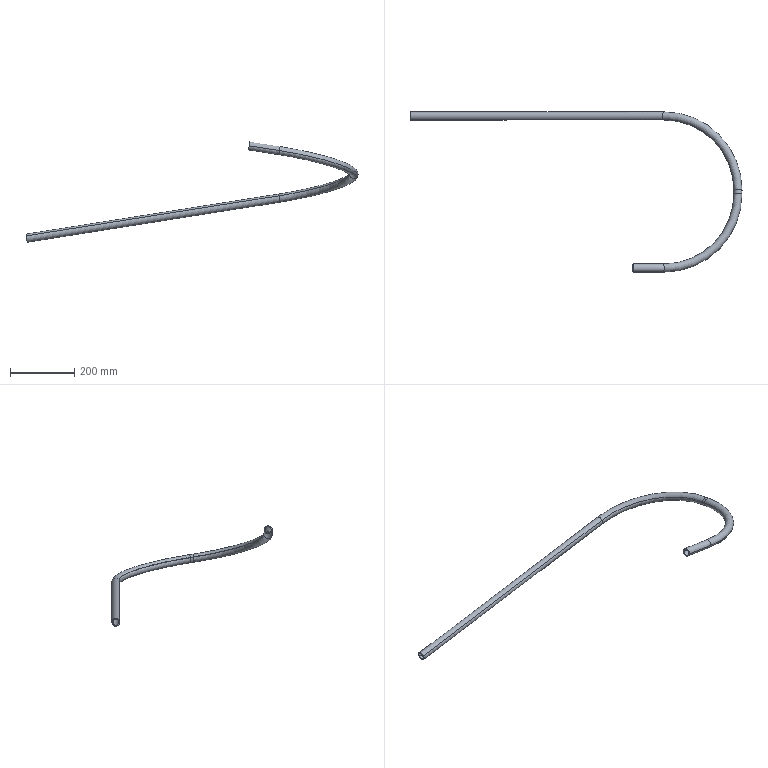Part | STEP file | 31E-01143WG10 | 1 solid | 22 faces | box 1031 x 498.4 x 311.784 mm | volume 326544 mm3 | cylinder 12 | torus 8 | plane 2 | commonest cylinder face diameters 19.8 x6 25.4 x6
STEP:
#1=CARTESIAN_POINT('',(-1196.479,198.036,1339.737));
#2=VERTEX_POINT('',#1);
#3=CARTESIAN_POINT('',(-411.266,198.036,1464.102));
#4=VERTEX_POINT('',#3);
#5=CARTESIAN_POINT('',(-427.761,198.036,1461.49));
#6=DIRECTION('',(0.9877,0.,0.1564));
#7=VECTOR('',#6,1.);
#8=LINE('',#5,#7);
#9=EDGE_CURVE('',#2,#4,#8,.T.);
#10=ORIENTED_EDGE('',*,*,#9,.F.);
#11=CARTESIAN_POINT('',(-1194.685,214.176,1328.409));
#12=VERTEX_POINT('',#11);
#13=CARTESIAN_POINT('',(-1195.582,206.106,1334.073));
#14=DIRECTION('',(0.9877,0.,0.1564));
#15=AXIS2_PLACEMENT_3D('',#13,#14,$);
#16=CIRCLE('',#15,9.9);
#17=EDGE_CURVE('',#2,#12,#16,.F.);
#18=ORIENTED_EDGE('',*,*,#17,.T.);
#19=CARTESIAN_POINT('',(-409.472,214.176,1452.774));
#20=VERTEX_POINT('',#19);
#21=CARTESIAN_POINT('',(-425.967,214.176,1450.162));
#22=DIRECTION('',(0.9877,0.,0.1564));
#23=VECTOR('',#22,1.);
#24=LINE('',#21,#23);
#25=EDGE_CURVE('',#12,#20,#24,.T.);
#26=ORIENTED_EDGE('',*,*,#25,.T.);
#27=CARTESIAN_POINT('',(-410.369,206.106,1458.438));
#28=DIRECTION('',(0.9877,0.,0.1564));
#29=AXIS2_PLACEMENT_3D('',#27,#28,$);
#30=CIRCLE('',#29,9.9);
#31=EDGE_CURVE('',#20,#4,#30,.T.);
#32=ORIENTED_EDGE('',*,*,#31,.T.);
#33=EDGE_LOOP('',(#10,#18,#26,#32));
#34=FACE_OUTER_BOUND('',#33,.T.);
#35=CARTESIAN_POINT('',(-426.864,206.106,1455.826));
#36=DIRECTION('',(0.9877,0.,0.1564));
#37=DIRECTION('',(0.09062,0.8151,-0.5721));
#38=AXIS2_PLACEMENT_3D('',#35,#36,#37);
#39=CYLINDRICAL_SURFACE('',#38,9.9);
#40=ADVANCED_FACE('',(#34),#39,.F.);
#41=CARTESIAN_POINT('',(-169.572,-25.868,1528.434));
#42=VERTEX_POINT('',#41);
#43=CARTESIAN_POINT('',(-415.434,-31.741,1490.415));
#44=DIRECTION('',(-0.1546,0.1531,0.976));
#45=AXIS2_PLACEMENT_3D('',#43,#44,$);
#46=CIRCLE('',#45,248.853);
#47=EDGE_CURVE('',#42,#20,#46,.T.);
#48=ORIENTED_EDGE('',*,*,#47,.F.);
#49=CARTESIAN_POINT('',(-188.435,-24.929,1534.379));
#50=VERTEX_POINT('',#49);
#51=CARTESIAN_POINT('',(-179.004,-25.399,1531.407));
#52=DIRECTION('',(-0.0003622,-0.9879,0.155));
#53=AXIS2_PLACEMENT_3D('',#51,#52,$);
#54=CIRCLE('',#53,9.9);
#55=EDGE_CURVE('',#42,#50,#54,.T.);
#56=ORIENTED_EDGE('',*,*,#55,.T.);
#57=CARTESIAN_POINT('',(-416.804,-30.384,1499.065));
#58=DIRECTION('',(-0.1546,0.1531,0.976));
#59=AXIS2_PLACEMENT_3D('',#57,#58,$);
#60=CIRCLE('',#59,231.147);
#61=EDGE_CURVE('',#50,#4,#60,.T.);
#62=ORIENTED_EDGE('',*,*,#61,.T.);
#63=ORIENTED_EDGE('',*,*,#31,.F.);
#64=EDGE_LOOP('',(#48,#56,#62,#63));
#65=FACE_OUTER_BOUND('',#64,.T.);
#66=CARTESIAN_POINT('',(-416.119,-31.063,1494.74));
#67=DIRECTION('',(-0.1546,0.1531,0.976));
#68=DIRECTION('',(0.988,0.0236,0.1528));
#69=AXIS2_PLACEMENT_3D('',#66,#67,#68);
#70=TOROIDAL_SURFACE('',#69,240.,9.9);
#71=ADVANCED_FACE('',(#65),#70,.F.);
#72=CARTESIAN_POINT('',(-169.576,-36.024,1530.027));
#73=VERTEX_POINT('',#72);
#74=CARTESIAN_POINT('',(-169.574,-30.946,1529.231));
#75=DIRECTION('',(-0.0003622,-0.9879,0.155));
#76=VECTOR('',#75,1.);
#77=LINE('',#74,#76);
#78=EDGE_CURVE('',#73,#42,#77,.F.);
#79=ORIENTED_EDGE('',*,*,#78,.F.);
#80=CARTESIAN_POINT('',(-188.439,-35.085,1535.972));
#81=VERTEX_POINT('',#80);
#82=CARTESIAN_POINT('',(-179.007,-35.555,1533.));
#83=DIRECTION('',(-0.0003622,-0.9879,0.155));
#84=AXIS2_PLACEMENT_3D('',#82,#83,$);
#85=CIRCLE('',#84,9.9);
#86=EDGE_CURVE('',#73,#81,#85,.T.);
#87=ORIENTED_EDGE('',*,*,#86,.T.);
#88=CARTESIAN_POINT('',(-188.437,-30.007,1535.176));
#89=DIRECTION('',(-0.0003622,-0.9879,0.155));
#90=VECTOR('',#89,1.);
#91=LINE('',#88,#90);
#92=EDGE_CURVE('',#81,#50,#91,.F.);
#93=ORIENTED_EDGE('',*,*,#92,.T.);
#94=ORIENTED_EDGE('',*,*,#55,.F.);
#95=EDGE_LOOP('',(#79,#87,#93,#94));
#96=FACE_OUTER_BOUND('',#95,.T.);
#97=CARTESIAN_POINT('',(-179.006,-30.477,1532.203));
#98=DIRECTION('',(-0.0003622,-0.9879,0.155));
#99=DIRECTION('',(0.9527,-0.04744,-0.3002));
#100=AXIS2_PLACEMENT_3D('',#97,#98,#99);
#101=CYLINDRICAL_SURFACE('',#100,9.9);
#102=ADVANCED_FACE('',(#96),#101,.F.);
#103=ORIENTED_EDGE('',*,*,#92,.F.);
#104=CARTESIAN_POINT('',(-179.007,-35.555,1533.));
#105=DIRECTION('',(-0.0003622,-0.9879,0.155));
#106=AXIS2_PLACEMENT_3D('',#104,#105,$);
#107=CIRCLE('',#106,9.9);
#108=EDGE_CURVE('',#81,#73,#107,.T.);
#109=ORIENTED_EDGE('',*,*,#108,.T.);
#110=ORIENTED_EDGE('',*,*,#78,.T.);
#111=CARTESIAN_POINT('',(-179.004,-25.399,1531.407));
#112=DIRECTION('',(-0.0003622,-0.9879,0.155));
#113=AXIS2_PLACEMENT_3D('',#111,#112,$);
#114=CIRCLE('',#113,9.9);
#115=EDGE_CURVE('',#50,#42,#114,.T.);
#116=ORIENTED_EDGE('',*,*,#115,.F.);
#117=EDGE_LOOP('',(#103,#109,#110,#116));
#118=FACE_OUTER_BOUND('',#117,.T.);
#119=CARTESIAN_POINT('',(-179.006,-30.477,1532.203));
#120=DIRECTION('',(-0.0003622,-0.9879,0.155));
#121=DIRECTION('',(-0.9527,0.04744,0.3002));
#122=AXIS2_PLACEMENT_3D('',#119,#120,#121);
#123=CYLINDRICAL_SURFACE('',#122,9.9);
#124=ADVANCED_FACE('',(#118),#123,.F.);
#125=CARTESIAN_POINT('',(-410.377,-256.994,1605.916));
#126=VERTEX_POINT('',#125);
#127=CARTESIAN_POINT('',(-410.377,-276.794,1605.916));
#128=VERTEX_POINT('',#127);
#129=CARTESIAN_POINT('',(-410.377,-266.894,1605.916));
#130=DIRECTION('',(0.9877,0.,-0.1564));
#131=AXIS2_PLACEMENT_3D('',#129,#130,$);
#132=CIRCLE('',#131,9.9);
#133=EDGE_CURVE('',#126,#128,#132,.F.);
#134=ORIENTED_EDGE('',*,*,#133,.T.);
#135=CARTESIAN_POINT('',(-416.356,-29.953,1568.162));
#136=DIRECTION('',(-0.1546,-0.153,-0.9761));
#137=AXIS2_PLACEMENT_3D('',#135,#136,$);
#138=CIRCLE('',#137,249.783);
#139=EDGE_CURVE('',#73,#128,#138,.T.);
#140=ORIENTED_EDGE('',*,*,#139,.F.);
#141=ORIENTED_EDGE('',*,*,#108,.F.);
#142=CARTESIAN_POINT('',(-415.888,-29.489,1571.119));
#143=DIRECTION('',(-0.1546,-0.153,-0.9761));
#144=AXIS2_PLACEMENT_3D('',#142,#143,$);
#145=CIRCLE('',#144,230.217);
#146=EDGE_CURVE('',#81,#126,#145,.T.);
#147=ORIENTED_EDGE('',*,*,#146,.T.);
#148=EDGE_LOOP('',(#134,#140,#141,#147));
#149=FACE_OUTER_BOUND('',#148,.T.);
#150=CARTESIAN_POINT('',(-416.122,-29.721,1569.64));
#151=DIRECTION('',(-0.1546,-0.153,-0.9761));
#152=DIRECTION('',(0.988,-0.02431,-0.1527));
#153=AXIS2_PLACEMENT_3D('',#150,#151,#152);
#154=TOROIDAL_SURFACE('',#153,240.,9.9);
#155=ADVANCED_FACE('',(#149),#154,.F.);
#156=CARTESIAN_POINT('',(-410.377,-266.894,1605.916));
#157=DIRECTION('',(0.9877,0.,-0.1564));
#158=AXIS2_PLACEMENT_3D('',#156,#157,$);
#159=CIRCLE('',#158,9.9);
#160=EDGE_CURVE('',#128,#126,#159,.F.);
#161=ORIENTED_EDGE('',*,*,#160,.T.);
#162=ORIENTED_EDGE('',*,*,#146,.F.);
#163=ORIENTED_EDGE('',*,*,#86,.F.);
#164=ORIENTED_EDGE('',*,*,#139,.T.);
#165=EDGE_LOOP('',(#161,#162,#163,#164));
#166=FACE_OUTER_BOUND('',#165,.T.);
#167=CARTESIAN_POINT('',(-416.122,-29.721,1569.64));
#168=DIRECTION('',(-0.1546,-0.153,-0.9761));
#169=DIRECTION('',(0.988,-0.02431,-0.1527));
#170=AXIS2_PLACEMENT_3D('',#167,#168,#169);
#171=TOROIDAL_SURFACE('',#170,240.,9.9);
#172=ADVANCED_FACE('',(#166),#171,.F.);
#173=CARTESIAN_POINT('',(-504.155,-276.794,1620.769));
#174=VERTEX_POINT('',#173);
#175=CARTESIAN_POINT('',(-433.907,-276.794,1609.643));
#176=DIRECTION('',(-0.9877,0.,0.1564));
#177=VECTOR('',#176,1.);
#178=LINE('',#175,#177);
#179=EDGE_CURVE('',#128,#174,#178,.T.);
#180=ORIENTED_EDGE('',*,*,#179,.T.);
#181=CARTESIAN_POINT('',(-504.155,-256.994,1620.769));
#182=VERTEX_POINT('',#181);
#183=CARTESIAN_POINT('',(-504.155,-266.894,1620.769));
#184=DIRECTION('',(-0.9877,0.,0.1564));
#185=AXIS2_PLACEMENT_3D('',#183,#184,$);
#186=CIRCLE('',#185,9.9);
#187=EDGE_CURVE('',#174,#182,#186,.T.);
#188=ORIENTED_EDGE('',*,*,#187,.T.);
#189=CARTESIAN_POINT('',(-433.907,-256.994,1609.643));
#190=DIRECTION('',(-0.9877,0.,0.1564));
#191=VECTOR('',#190,1.);
#192=LINE('',#189,#191);
#193=EDGE_CURVE('',#126,#182,#192,.T.);
#194=ORIENTED_EDGE('',*,*,#193,.F.);
#195=ORIENTED_EDGE('',*,*,#160,.F.);
#196=EDGE_LOOP('',(#180,#188,#194,#195));
#197=FACE_OUTER_BOUND('',#196,.T.);
#198=CARTESIAN_POINT('',(-433.907,-266.894,1609.643));
#199=DIRECTION('',(-0.9877,0.,0.1564));
#200=DIRECTION('',(0.,-1.,0.));
#201=AXIS2_PLACEMENT_3D('',#198,#199,#200);
#202=CYLINDRICAL_SURFACE('',#201,9.9);
#203=ADVANCED_FACE('',(#197),#202,.F.);
#204=CARTESIAN_POINT('',(-504.155,-266.894,1620.769));
#205=DIRECTION('',(-0.9877,0.,0.1564));
#206=AXIS2_PLACEMENT_3D('',#204,#205,$);
#207=CIRCLE('',#206,9.9);
#208=EDGE_CURVE('',#182,#174,#207,.T.);
#209=ORIENTED_EDGE('',*,*,#208,.T.);
#210=ORIENTED_EDGE('',*,*,#179,.F.);
#211=ORIENTED_EDGE('',*,*,#133,.F.);
#212=ORIENTED_EDGE('',*,*,#193,.T.);
#213=EDGE_LOOP('',(#209,#210,#211,#212));
#214=FACE_OUTER_BOUND('',#213,.T.);
#215=CARTESIAN_POINT('',(-433.907,-266.894,1609.643));
#216=DIRECTION('',(-0.9877,0.,0.1564));
#217=DIRECTION('',(0.,1.,0.));
#218=AXIS2_PLACEMENT_3D('',#215,#216,#217);
#219=CYLINDRICAL_SURFACE('',#218,9.9);
#220=ADVANCED_FACE('',(#214),#219,.F.);
#221=CARTESIAN_POINT('',(-504.155,-254.194,1620.769));
#222=VERTEX_POINT('',#221);
#223=CARTESIAN_POINT('',(-504.155,-279.594,1620.769));
#224=VERTEX_POINT('',#223);
#225=CARTESIAN_POINT('',(-504.155,-279.594,1620.769));
#226=CARTESIAN_POINT('',(-504.467,-279.594,1618.799));
#227=CARTESIAN_POINT('',(-504.779,-279.202,1616.828));
#228=CARTESIAN_POINT('',(-505.075,-278.418,1614.959));
#229=CARTESIAN_POINT('',(-505.603,-276.151,1611.626));
#230=CARTESIAN_POINT('',(-505.958,-272.776,1609.386));
#231=CARTESIAN_POINT('',(-506.081,-270.884,1608.612));
#232=CARTESIAN_POINT('',(-506.203,-266.894,1607.839));
#233=CARTESIAN_POINT('',(-506.081,-262.904,1608.612));
#234=CARTESIAN_POINT('',(-505.958,-261.012,1609.386));
#235=CARTESIAN_POINT('',(-505.603,-257.637,1611.626));
#236=CARTESIAN_POINT('',(-505.075,-255.369,1614.959));
#237=CARTESIAN_POINT('',(-504.779,-254.586,1616.828));
#238=CARTESIAN_POINT('',(-504.467,-254.194,1618.799));
#239=CARTESIAN_POINT('',(-504.155,-254.194,1620.769));
#240=B_SPLINE_CURVE_WITH_KNOTS('',5,(#225,#226,#227,#228,#229,#230,#231,#232,#233,#234,#235,#236,#237,#238,#239),.UNSPECIFIED.,.F.,.U.,(6,3,3,3,6),(39.898,49.873,59.847,69.822,79.796),.UNSPECIFIED.);
#241=EDGE_CURVE('',#222,#224,#240,.F.);
#242=ORIENTED_EDGE('',*,*,#241,.T.);
#243=CARTESIAN_POINT('',(-504.155,-254.194,1620.769));
#244=CARTESIAN_POINT('',(-503.843,-254.194,1622.739));
#245=CARTESIAN_POINT('',(-503.531,-254.586,1624.71));
#246=CARTESIAN_POINT('',(-503.235,-255.369,1626.579));
#247=CARTESIAN_POINT('',(-502.707,-257.637,1629.912));
#248=CARTESIAN_POINT('',(-502.352,-261.012,1632.152));
#249=CARTESIAN_POINT('',(-502.23,-262.904,1632.926));
#250=CARTESIAN_POINT('',(-502.107,-266.894,1633.7));
#251=CARTESIAN_POINT('',(-502.23,-270.884,1632.926));
#252=CARTESIAN_POINT('',(-502.352,-272.776,1632.152));
#253=CARTESIAN_POINT('',(-502.707,-276.151,1629.912));
#254=CARTESIAN_POINT('',(-503.235,-278.418,1626.579));
#255=CARTESIAN_POINT('',(-503.531,-279.202,1624.71));
#256=CARTESIAN_POINT('',(-503.843,-279.594,1622.739));
#257=CARTESIAN_POINT('',(-504.155,-279.594,1620.769));
#258=B_SPLINE_CURVE_WITH_KNOTS('',5,(#243,#244,#245,#246,#247,#248,#249,#250,#251,#252,#253,#254,#255,#256,#257),.UNSPECIFIED.,.F.,.U.,(6,3,3,3,6),(0.,9.975,19.949,29.924,39.898),.UNSPECIFIED.);
#259=EDGE_CURVE('',#224,#222,#258,.F.);
#260=ORIENTED_EDGE('',*,*,#259,.T.);
#261=EDGE_LOOP('',(#242,#260));
#262=FACE_OUTER_BOUND('',#261,.T.);
#263=ORIENTED_EDGE('',*,*,#208,.F.);
#264=ORIENTED_EDGE('',*,*,#187,.F.);
#265=EDGE_LOOP('',(#263,#264));
#266=FACE_BOUND('',#265,.T.);
#267=CARTESIAN_POINT('',(-504.155,-266.894,1620.769));
#268=DIRECTION('',(0.9877,0.,-0.1564));
#269=DIRECTION('',(0.,1.,0.));
#270=AXIS2_PLACEMENT_3D('',#267,#268,#269);
#271=PLANE('',#270);
#272=ADVANCED_FACE('',(#262,#266),#271,.F.);
#273=CARTESIAN_POINT('',(-410.377,-279.594,1605.916));
#274=VERTEX_POINT('',#273);
#275=CARTESIAN_POINT('',(-433.907,-279.594,1609.643));
#276=DIRECTION('',(-0.9877,0.,0.1564));
#277=VECTOR('',#276,1.);
#278=LINE('',#275,#277);
#279=EDGE_CURVE('',#274,#224,#278,.T.);
#280=ORIENTED_EDGE('',*,*,#279,.F.);
#281=CARTESIAN_POINT('',(-410.377,-254.194,1605.916));
#282=VERTEX_POINT('',#281);
#283=CARTESIAN_POINT('',(-410.377,-266.894,1605.916));
#284=DIRECTION('',(-0.9877,0.,0.1564));
#285=AXIS2_PLACEMENT_3D('',#283,#284,$);
#286=CIRCLE('',#285,12.7);
#287=EDGE_CURVE('',#274,#282,#286,.T.);
#288=ORIENTED_EDGE('',*,*,#287,.T.);
#289=CARTESIAN_POINT('',(-433.907,-254.194,1609.643));
#290=DIRECTION('',(-0.9877,0.,0.1564));
#291=VECTOR('',#290,1.);
#292=LINE('',#289,#291);
#293=EDGE_CURVE('',#282,#222,#292,.T.);
#294=ORIENTED_EDGE('',*,*,#293,.T.);
#295=ORIENTED_EDGE('',*,*,#259,.F.);
#296=EDGE_LOOP('',(#280,#288,#294,#295));
#297=FACE_OUTER_BOUND('',#296,.T.);
#298=CARTESIAN_POINT('',(-433.907,-266.894,1609.643));
#299=DIRECTION('',(-0.9877,0.,0.1564));
#300=DIRECTION('',(0.,-1.,0.));
#301=AXIS2_PLACEMENT_3D('',#298,#299,#300);
#302=CYLINDRICAL_SURFACE('',#301,12.7);
#303=ADVANCED_FACE('',(#297),#302,.T.);
#304=CARTESIAN_POINT('',(-166.908,-36.157,1529.187));
#305=VERTEX_POINT('',#304);
#306=CARTESIAN_POINT('',(-416.423,-30.018,1567.743));
#307=DIRECTION('',(-0.1546,-0.153,-0.9761));
#308=AXIS2_PLACEMENT_3D('',#306,#307,$);
#309=CIRCLE('',#308,252.55);
#310=EDGE_CURVE('',#305,#274,#309,.T.);
#311=ORIENTED_EDGE('',*,*,#310,.F.);
#312=CARTESIAN_POINT('',(-191.107,-34.952,1536.813));
#313=VERTEX_POINT('',#312);
#314=CARTESIAN_POINT('',(-179.007,-35.555,1533.));
#315=DIRECTION('',(0.0003622,0.9879,-0.155));
#316=AXIS2_PLACEMENT_3D('',#314,#315,$);
#317=CIRCLE('',#316,12.7);
#318=EDGE_CURVE('',#305,#313,#317,.F.);
#319=ORIENTED_EDGE('',*,*,#318,.T.);
#320=CARTESIAN_POINT('',(-415.822,-29.423,1571.537));
#321=DIRECTION('',(-0.1546,-0.153,-0.9761));
#322=AXIS2_PLACEMENT_3D('',#320,#321,$);
#323=CIRCLE('',#322,227.45);
#324=EDGE_CURVE('',#313,#282,#323,.T.);
#325=ORIENTED_EDGE('',*,*,#324,.T.);
#326=ORIENTED_EDGE('',*,*,#287,.F.);
#327=EDGE_LOOP('',(#311,#319,#325,#326));
#328=FACE_OUTER_BOUND('',#327,.T.);
#329=CARTESIAN_POINT('',(-416.122,-29.721,1569.64));
#330=DIRECTION('',(-0.1546,-0.153,-0.9761));
#331=DIRECTION('',(0.988,-0.02431,-0.1527));
#332=AXIS2_PLACEMENT_3D('',#329,#330,#331);
#333=TOROIDAL_SURFACE('',#332,240.,12.7);
#334=ADVANCED_FACE('',(#328),#333,.T.);
#335=CARTESIAN_POINT('',(-166.905,-26.001,1527.594));
#336=VERTEX_POINT('',#335);
#337=CARTESIAN_POINT('',(-191.103,-24.796,1535.22));
#338=VERTEX_POINT('',#337);
#339=CARTESIAN_POINT('',(-179.004,-25.399,1531.407));
#340=DIRECTION('',(-0.0003622,-0.9879,0.155));
#341=AXIS2_PLACEMENT_3D('',#339,#340,$);
#342=CIRCLE('',#341,12.7);
#343=EDGE_CURVE('',#336,#338,#342,.T.);
#344=ORIENTED_EDGE('',*,*,#343,.T.);
#345=CARTESIAN_POINT('',(-191.105,-29.874,1536.016));
#346=DIRECTION('',(-0.0003622,-0.9879,0.155));
#347=VECTOR('',#346,1.);
#348=LINE('',#345,#347);
#349=EDGE_CURVE('',#313,#338,#348,.F.);
#350=ORIENTED_EDGE('',*,*,#349,.F.);
#351=ORIENTED_EDGE('',*,*,#318,.F.);
#352=CARTESIAN_POINT('',(-166.906,-31.079,1528.39));
#353=DIRECTION('',(-0.0003622,-0.9879,0.155));
#354=VECTOR('',#353,1.);
#355=LINE('',#352,#354);
#356=EDGE_CURVE('',#305,#336,#355,.F.);
#357=ORIENTED_EDGE('',*,*,#356,.T.);
#358=EDGE_LOOP('',(#344,#350,#351,#357));
#359=FACE_OUTER_BOUND('',#358,.T.);
#360=CARTESIAN_POINT('',(-179.006,-30.477,1532.203));
#361=DIRECTION('',(-0.0003622,-0.9879,0.155));
#362=DIRECTION('',(0.9527,-0.04744,-0.3002));
#363=AXIS2_PLACEMENT_3D('',#360,#361,#362);
#364=CYLINDRICAL_SURFACE('',#363,12.7);
#365=ADVANCED_FACE('',(#359),#364,.T.);
#366=CARTESIAN_POINT('',(-179.004,-25.399,1531.407));
#367=DIRECTION('',(-0.0003622,-0.9879,0.155));
#368=AXIS2_PLACEMENT_3D('',#366,#367,$);
#369=CIRCLE('',#368,12.7);
#370=EDGE_CURVE('',#338,#336,#369,.T.);
#371=ORIENTED_EDGE('',*,*,#370,.T.);
#372=ORIENTED_EDGE('',*,*,#356,.F.);
#373=CARTESIAN_POINT('',(-179.007,-35.555,1533.));
#374=DIRECTION('',(-0.0003622,-0.9879,0.155));
#375=AXIS2_PLACEMENT_3D('',#373,#374,$);
#376=CIRCLE('',#375,12.7);
#377=EDGE_CURVE('',#313,#305,#376,.T.);
#378=ORIENTED_EDGE('',*,*,#377,.F.);
#379=ORIENTED_EDGE('',*,*,#349,.T.);
#380=EDGE_LOOP('',(#371,#372,#378,#379));
#381=FACE_OUTER_BOUND('',#380,.T.);
#382=CARTESIAN_POINT('',(-179.006,-30.477,1532.203));
#383=DIRECTION('',(-0.0003622,-0.9879,0.155));
#384=DIRECTION('',(-0.9527,0.04744,0.3002));
#385=AXIS2_PLACEMENT_3D('',#382,#383,#384);
#386=CYLINDRICAL_SURFACE('',#385,12.7);
#387=ADVANCED_FACE('',(#381),#386,.T.);
#388=ORIENTED_EDGE('',*,*,#324,.F.);
#389=ORIENTED_EDGE('',*,*,#377,.T.);
#390=ORIENTED_EDGE('',*,*,#310,.T.);
#391=CARTESIAN_POINT('',(-410.377,-266.894,1605.916));
#392=DIRECTION('',(0.9877,0.,-0.1564));
#393=AXIS2_PLACEMENT_3D('',#391,#392,$);
#394=CIRCLE('',#393,12.7);
#395=EDGE_CURVE('',#282,#274,#394,.F.);
#396=ORIENTED_EDGE('',*,*,#395,.F.);
#397=EDGE_LOOP('',(#388,#389,#390,#396));
#398=FACE_OUTER_BOUND('',#397,.T.);
#399=CARTESIAN_POINT('',(-416.122,-29.721,1569.64));
#400=DIRECTION('',(-0.1546,-0.153,-0.9761));
#401=DIRECTION('',(0.988,-0.02431,-0.1527));
#402=AXIS2_PLACEMENT_3D('',#399,#400,#401);
#403=TOROIDAL_SURFACE('',#402,240.,12.7);
#404=ADVANCED_FACE('',(#398),#403,.T.);
#405=ORIENTED_EDGE('',*,*,#279,.T.);
#406=ORIENTED_EDGE('',*,*,#241,.F.);
#407=ORIENTED_EDGE('',*,*,#293,.F.);
#408=ORIENTED_EDGE('',*,*,#395,.T.);
#409=EDGE_LOOP('',(#405,#406,#407,#408));
#410=FACE_OUTER_BOUND('',#409,.T.);
#411=CARTESIAN_POINT('',(-433.907,-266.894,1609.643));
#412=DIRECTION('',(-0.9877,0.,0.1564));
#413=DIRECTION('',(0.,1.,0.));
#414=AXIS2_PLACEMENT_3D('',#411,#412,#413);
#415=CYLINDRICAL_SURFACE('',#414,12.7);
#416=ADVANCED_FACE('',(#410),#415,.T.);
#417=CARTESIAN_POINT('',(-411.52,195.754,1465.704));
#418=VERTEX_POINT('',#417);
#419=CARTESIAN_POINT('',(-409.218,216.458,1451.172));
#420=VERTEX_POINT('',#419);
#421=CARTESIAN_POINT('',(-410.369,206.106,1458.438));
#422=DIRECTION('',(0.9877,0.,0.1564));
#423=AXIS2_PLACEMENT_3D('',#421,#422,$);
#424=CIRCLE('',#423,12.7);
#425=EDGE_CURVE('',#418,#420,#424,.T.);
#426=ORIENTED_EDGE('',*,*,#425,.T.);
#427=CARTESIAN_POINT('',(-415.24,-31.933,1489.192));
#428=DIRECTION('',(-0.1546,0.1531,0.976));
#429=AXIS2_PLACEMENT_3D('',#427,#428,$);
#430=CIRCLE('',#429,251.357);
#431=EDGE_CURVE('',#336,#420,#430,.T.);
#432=ORIENTED_EDGE('',*,*,#431,.F.);
#433=ORIENTED_EDGE('',*,*,#370,.F.);
#434=CARTESIAN_POINT('',(-416.997,-30.192,1500.288));
#435=DIRECTION('',(-0.1546,0.1531,0.976));
#436=AXIS2_PLACEMENT_3D('',#434,#435,$);
#437=CIRCLE('',#436,228.643);
#438=EDGE_CURVE('',#338,#418,#437,.T.);
#439=ORIENTED_EDGE('',*,*,#438,.T.);
#440=EDGE_LOOP('',(#426,#432,#433,#439));
#441=FACE_OUTER_BOUND('',#440,.T.);
#442=CARTESIAN_POINT('',(-416.119,-31.063,1494.74));
#443=DIRECTION('',(-0.1546,0.1531,0.976));
#444=DIRECTION('',(0.988,0.0236,0.1528));
#445=AXIS2_PLACEMENT_3D('',#442,#443,#444);
#446=TOROIDAL_SURFACE('',#445,240.,12.7);
#447=ADVANCED_FACE('',(#441),#446,.T.);
#448=CARTESIAN_POINT('',(-410.369,206.106,1458.438));
#449=DIRECTION('',(0.9877,0.,0.1564));
#450=AXIS2_PLACEMENT_3D('',#448,#449,$);
#451=CIRCLE('',#450,12.7);
#452=EDGE_CURVE('',#420,#418,#451,.T.);
#453=ORIENTED_EDGE('',*,*,#452,.T.);
#454=ORIENTED_EDGE('',*,*,#438,.F.);
#455=ORIENTED_EDGE('',*,*,#343,.F.);
#456=ORIENTED_EDGE('',*,*,#431,.T.);
#457=EDGE_LOOP('',(#453,#454,#455,#456));
#458=FACE_OUTER_BOUND('',#457,.T.);
#459=CARTESIAN_POINT('',(-416.119,-31.063,1494.74));
#460=DIRECTION('',(-0.1546,0.1531,0.976));
#461=DIRECTION('',(0.988,0.0236,0.1528));
#462=AXIS2_PLACEMENT_3D('',#459,#460,#461);
#463=TOROIDAL_SURFACE('',#462,240.,12.7);
#464=ADVANCED_FACE('',(#458),#463,.T.);
#465=ORIENTED_EDGE('',*,*,#452,.F.);
#466=CARTESIAN_POINT('',(-1194.431,216.458,1326.807));
#467=VERTEX_POINT('',#466);
#468=CARTESIAN_POINT('',(-425.713,216.458,1448.56));
#469=DIRECTION('',(0.9877,0.,0.1564));
#470=VECTOR('',#469,1.);
#471=LINE('',#468,#470);
#472=EDGE_CURVE('',#467,#420,#471,.T.);
#473=ORIENTED_EDGE('',*,*,#472,.F.);
#474=CARTESIAN_POINT('',(-1196.733,195.754,1341.339));
#475=VERTEX_POINT('',#474);
#476=CARTESIAN_POINT('',(-1195.582,206.106,1334.073));
#477=DIRECTION('',(0.9877,0.,0.1564));
#478=AXIS2_PLACEMENT_3D('',#476,#477,$);
#479=CIRCLE('',#478,12.7);
#480=EDGE_CURVE('',#475,#467,#479,.F.);
#481=ORIENTED_EDGE('',*,*,#480,.F.);
#482=CARTESIAN_POINT('',(-428.015,195.754,1463.092));
#483=DIRECTION('',(0.9877,0.,0.1564));
#484=VECTOR('',#483,1.);
#485=LINE('',#482,#484);
#486=EDGE_CURVE('',#475,#418,#485,.T.);
#487=ORIENTED_EDGE('',*,*,#486,.T.);
#488=EDGE_LOOP('',(#465,#473,#481,#487));
#489=FACE_OUTER_BOUND('',#488,.T.);
#490=CARTESIAN_POINT('',(-426.864,206.106,1455.826));
#491=DIRECTION('',(0.9877,0.,0.1564));
#492=DIRECTION('',(0.09062,0.8151,-0.5721));
#493=AXIS2_PLACEMENT_3D('',#490,#491,#492);
#494=CYLINDRICAL_SURFACE('',#493,12.7);
#495=ADVANCED_FACE('',(#489),#494,.T.);
#496=ORIENTED_EDGE('',*,*,#486,.F.);
#497=CARTESIAN_POINT('',(-1195.582,206.106,1334.073));
#498=DIRECTION('',(0.9877,0.,0.1564));
#499=AXIS2_PLACEMENT_3D('',#497,#498,$);
#500=CIRCLE('',#499,12.7);
#501=EDGE_CURVE('',#467,#475,#500,.F.);
#502=ORIENTED_EDGE('',*,*,#501,.F.);
#503=ORIENTED_EDGE('',*,*,#472,.T.);
#504=ORIENTED_EDGE('',*,*,#425,.F.);
#505=EDGE_LOOP('',(#496,#502,#503,#504));
#506=FACE_OUTER_BOUND('',#505,.T.);
#507=CARTESIAN_POINT('',(-426.864,206.106,1455.826));
#508=DIRECTION('',(0.9877,0.,0.1564));
#509=DIRECTION('',(-0.09062,-0.8151,0.5721));
#510=AXIS2_PLACEMENT_3D('',#507,#508,#509);
#511=CYLINDRICAL_SURFACE('',#510,12.7);
#512=ADVANCED_FACE('',(#506),#511,.T.);
#513=ORIENTED_EDGE('',*,*,#501,.T.);
#514=ORIENTED_EDGE('',*,*,#480,.T.);
#515=EDGE_LOOP('',(#513,#514));
#516=FACE_OUTER_BOUND('',#515,.T.);
#517=ORIENTED_EDGE('',*,*,#17,.F.);
#518=CARTESIAN_POINT('',(-1196.479,198.036,1339.737));
#519=CARTESIAN_POINT('',(-1196.281,197.135,1338.485));
#520=CARTESIAN_POINT('',(-1196.055,196.483,1337.058));
#521=CARTESIAN_POINT('',(-1195.811,196.127,1335.521));
#522=CARTESIAN_POINT('',(-1195.316,196.044,1332.391));
#523=CARTESIAN_POINT('',(-1194.852,197.165,1329.463));
#524=CARTESIAN_POINT('',(-1194.64,198.013,1328.127));
#525=CARTESIAN_POINT('',(-1194.281,200.195,1325.856));
#526=CARTESIAN_POINT('',(-1194.077,203.084,1324.569));
#527=CARTESIAN_POINT('',(-1194.021,204.64,1324.217));
#528=CARTESIAN_POINT('',(-1194.008,207.808,1324.134));
#529=CARTESIAN_POINT('',(-1194.183,210.773,1325.241));
#530=CARTESIAN_POINT('',(-1194.316,212.126,1326.079));
#531=CARTESIAN_POINT('',(-1194.487,213.275,1327.157));
#532=CARTESIAN_POINT('',(-1194.685,214.176,1328.409));
#533=B_SPLINE_CURVE_WITH_KNOTS('',5,(#518,#519,#520,#521,#522,#523,#524,#525,#526,#527,#528,#529,#530,#531,#532),.UNSPECIFIED.,.F.,.U.,(6,3,3,3,6),(24.985,32.761,40.536,48.312,56.087),.UNSPECIFIED.);
#534=EDGE_CURVE('',#2,#12,#533,.T.);
#535=ORIENTED_EDGE('',*,*,#534,.T.);
#536=EDGE_LOOP('',(#517,#535));
#537=FACE_BOUND('',#536,.T.);
#538=CARTESIAN_POINT('',(-1195.582,206.106,1334.073));
#539=DIRECTION('',(0.9877,0.,0.1564));
#540=DIRECTION('',(0.,1.,0.));
#541=AXIS2_PLACEMENT_3D('',#538,#539,#540);
#542=PLANE('',#541);
#543=ADVANCED_FACE('',(#516,#537),#542,.F.);
#544=ORIENTED_EDGE('',*,*,#534,.F.);
#545=ORIENTED_EDGE('',*,*,#9,.T.);
#546=CARTESIAN_POINT('',(-410.369,206.106,1458.438));
#547=DIRECTION('',(0.9877,0.,0.1564));
#548=AXIS2_PLACEMENT_3D('',#546,#547,$);
#549=CIRCLE('',#548,9.9);
#550=EDGE_CURVE('',#4,#20,#549,.T.);
#551=ORIENTED_EDGE('',*,*,#550,.T.);
#552=ORIENTED_EDGE('',*,*,#25,.F.);
#553=EDGE_LOOP('',(#544,#545,#551,#552));
#554=FACE_OUTER_BOUND('',#553,.T.);
#555=CARTESIAN_POINT('',(-426.864,206.106,1455.826));
#556=DIRECTION('',(0.9877,0.,0.1564));
#557=DIRECTION('',(-0.09062,-0.8151,0.5721));
#558=AXIS2_PLACEMENT_3D('',#555,#556,#557);
#559=CYLINDRICAL_SURFACE('',#558,9.9);
#560=ADVANCED_FACE('',(#554),#559,.F.);
#561=ORIENTED_EDGE('',*,*,#61,.F.);
#562=ORIENTED_EDGE('',*,*,#115,.T.);
#563=ORIENTED_EDGE('',*,*,#47,.T.);
#564=ORIENTED_EDGE('',*,*,#550,.F.);
#565=EDGE_LOOP('',(#561,#562,#563,#564));
#566=FACE_OUTER_BOUND('',#565,.T.);
#567=CARTESIAN_POINT('',(-416.119,-31.063,1494.74));
#568=DIRECTION('',(-0.1546,0.1531,0.976));
#569=DIRECTION('',(0.988,0.0236,0.1528));
#570=AXIS2_PLACEMENT_3D('',#567,#568,#569);
#571=TOROIDAL_SURFACE('',#570,240.,9.9);
#572=ADVANCED_FACE('',(#566),#571,.F.);
#573=CLOSED_SHELL('',(#40,#71,#102,#124,#155,#172,#203,#220,#272,#303,#334,#365,#387,#404,#416,#447,#464,#495,#512,#543,#560,#572));
#574=MANIFOLD_SOLID_BREP('',#573);
#575=(LENGTH_UNIT()NAMED_UNIT(*)SI_UNIT(.MILLI.,.METRE.));
#576=UNCERTAINTY_MEASURE_WITH_UNIT(LENGTH_MEASURE(0.005),#575,'','');
#577=(NAMED_UNIT(*)PLANE_ANGLE_UNIT()SI_UNIT($,.RADIAN.));
#578=(NAMED_UNIT(*)SI_UNIT($,.STERADIAN.)SOLID_ANGLE_UNIT());
#579=(GEOMETRIC_REPRESENTATION_CONTEXT(3)GLOBAL_UNCERTAINTY_ASSIGNED_CONTEXT((#576))GLOBAL_UNIT_ASSIGNED_CONTEXT((#575,#577,#578))REPRESENTATION_CONTEXT('',''));
#580=ADVANCED_BREP_SHAPE_REPRESENTATION('',(#574),#579);